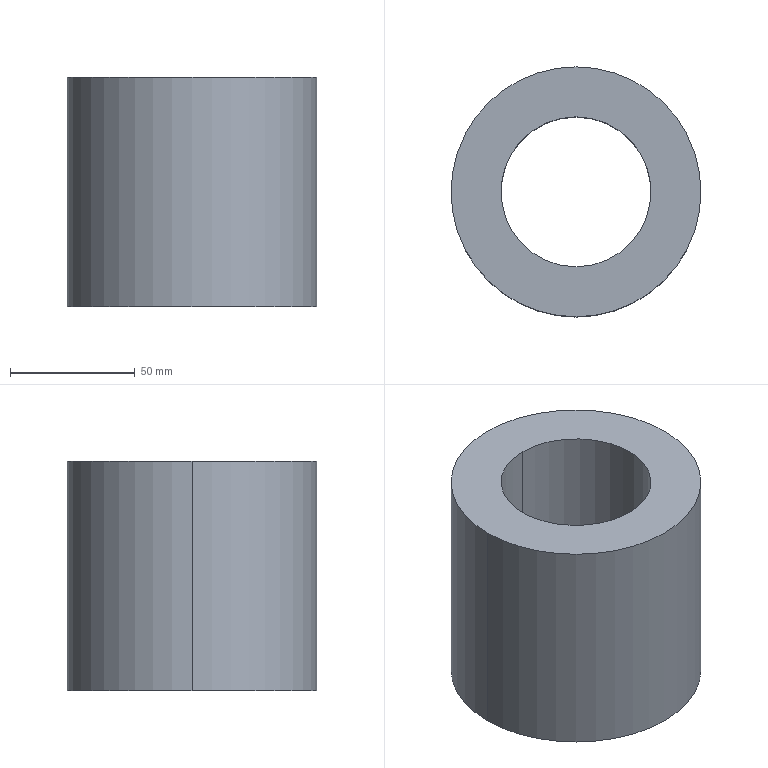Part | SolidWorks | features BaseBody 1 | 1 solid | 8 faces | box 100 x 100 x 92 mm | volume 462347 mm3 | cylinder 4 | cone 2 | plane 2 | commonest cylinder face diameters 60 x2 100 x2
STEP:
#1=CARTESIAN_POINT('',(0.,-30.,4.));
#2=VERTEX_POINT('',#1);
#3=CARTESIAN_POINT('',(0.,30.,4.));
#4=VERTEX_POINT('',#3);
#5=CARTESIAN_POINT('',(0.,0.,4.));
#6=DIRECTION('',(0.,0.,-1.));
#7=DIRECTION('',(0.,1.,0.));
#8=AXIS2_PLACEMENT_3D('',#5,#6,#7);
#9=CIRCLE('',#8,30.);
#10=EDGE_CURVE('',#2,#4,#9,.T.);
#11=ORIENTED_EDGE('',*,*,#10,.F.);
#12=CARTESIAN_POINT('',(0.,-31.,3.));
#13=VERTEX_POINT('',#12);
#14=CARTESIAN_POINT('',(0.,-30.,4.));
#15=DIRECTION('',(0.,-0.7071,-0.7071));
#16=VECTOR('',#15,1000.);
#17=LINE('',#14,#16);
#18=EDGE_CURVE('',#2,#13,#17,.T.);
#19=ORIENTED_EDGE('',*,*,#18,.T.);
#20=CARTESIAN_POINT('',(0.,31.,3.));
#21=VERTEX_POINT('',#20);
#22=CARTESIAN_POINT('',(0.,0.,3.));
#23=DIRECTION('',(0.,0.,1.));
#24=DIRECTION('',(0.,1.,0.));
#25=AXIS2_PLACEMENT_3D('',#22,#23,#24);
#26=CIRCLE('',#25,31.);
#27=EDGE_CURVE('',#21,#13,#26,.T.);
#28=ORIENTED_EDGE('',*,*,#27,.F.);
#29=CARTESIAN_POINT('',(0.,30.,4.));
#30=DIRECTION('',(0.,0.7071,-0.7071));
#31=VECTOR('',#30,1000.);
#32=LINE('',#29,#31);
#33=EDGE_CURVE('',#4,#21,#32,.T.);
#34=ORIENTED_EDGE('',*,*,#33,.F.);
#35=EDGE_LOOP('',(#11,#19,#28,#34));
#36=FACE_OUTER_BOUND('',#35,.T.);
#37=CARTESIAN_POINT('',(0.,0.,4.));
#38=DIRECTION('',(0.,0.,-1.));
#39=DIRECTION('',(0.,1.,0.));
#40=AXIS2_PLACEMENT_3D('',#37,#38,#39);
#41=CONICAL_SURFACE('',#40,30.,0.7854);
#42=ADVANCED_FACE('',(#36),#41,.F.);
#43=ORIENTED_EDGE('',*,*,#10,.T.);
#44=CARTESIAN_POINT('',(0.,30.,95.));
#45=VERTEX_POINT('',#44);
#46=CARTESIAN_POINT('',(0.,30.,-80.));
#47=DIRECTION('',(0.,0.,1.));
#48=VECTOR('',#47,1000.);
#49=LINE('',#46,#48);
#50=EDGE_CURVE('',#4,#45,#49,.T.);
#51=ORIENTED_EDGE('',*,*,#50,.T.);
#52=CARTESIAN_POINT('',(0.,-30.,95.));
#53=VERTEX_POINT('',#52);
#54=CARTESIAN_POINT('',(0.,0.,95.));
#55=DIRECTION('',(0.,0.,1.));
#56=DIRECTION('',(1.,0.,0.));
#57=AXIS2_PLACEMENT_3D('',#54,#55,#56);
#58=CIRCLE('',#57,30.);
#59=EDGE_CURVE('',#45,#53,#58,.T.);
#60=ORIENTED_EDGE('',*,*,#59,.T.);
#61=CARTESIAN_POINT('',(0.,-30.,-80.));
#62=DIRECTION('',(0.,0.,1.));
#63=VECTOR('',#62,1000.);
#64=LINE('',#61,#63);
#65=EDGE_CURVE('',#2,#53,#64,.T.);
#66=ORIENTED_EDGE('',*,*,#65,.F.);
#67=EDGE_LOOP('',(#43,#51,#60,#66));
#68=FACE_OUTER_BOUND('',#67,.T.);
#69=CARTESIAN_POINT('',(0.,0.,-80.));
#70=DIRECTION('',(0.,0.,1.));
#71=DIRECTION('',(0.,-1.,0.));
#72=AXIS2_PLACEMENT_3D('',#69,#70,#71);
#73=CYLINDRICAL_SURFACE('',#72,30.);
#74=ADVANCED_FACE('',(#68),#73,.F.);
#75=CARTESIAN_POINT('',(50.,0.,95.));
#76=VERTEX_POINT('',#75);
#77=CARTESIAN_POINT('',(-50.,0.,95.));
#78=VERTEX_POINT('',#77);
#79=CARTESIAN_POINT('',(0.,0.,95.));
#80=DIRECTION('',(0.,0.,1.));
#81=DIRECTION('',(1.,0.,0.));
#82=AXIS2_PLACEMENT_3D('',#79,#80,#81);
#83=CIRCLE('',#82,50.);
#84=EDGE_CURVE('',#76,#78,#83,.T.);
#85=ORIENTED_EDGE('',*,*,#84,.F.);
#86=CARTESIAN_POINT('',(50.,0.,3.));
#87=VERTEX_POINT('',#86);
#88=CARTESIAN_POINT('',(50.,0.,95.));
#89=DIRECTION('',(0.,0.,-1.));
#90=VECTOR('',#89,1000.);
#91=LINE('',#88,#90);
#92=EDGE_CURVE('',#76,#87,#91,.T.);
#93=ORIENTED_EDGE('',*,*,#92,.T.);
#94=CARTESIAN_POINT('',(-50.,0.,3.));
#95=VERTEX_POINT('',#94);
#96=CARTESIAN_POINT('',(0.,0.,3.));
#97=DIRECTION('',(0.,0.,-1.));
#98=DIRECTION('',(0.,1.,0.));
#99=AXIS2_PLACEMENT_3D('',#96,#97,#98);
#100=CIRCLE('',#99,50.);
#101=EDGE_CURVE('',#95,#87,#100,.T.);
#102=ORIENTED_EDGE('',*,*,#101,.F.);
#103=CARTESIAN_POINT('',(-50.,0.,95.));
#104=DIRECTION('',(0.,0.,-1.));
#105=VECTOR('',#104,1000.);
#106=LINE('',#103,#105);
#107=EDGE_CURVE('',#78,#95,#106,.T.);
#108=ORIENTED_EDGE('',*,*,#107,.F.);
#109=EDGE_LOOP('',(#85,#93,#102,#108));
#110=FACE_OUTER_BOUND('',#109,.T.);
#111=CARTESIAN_POINT('',(0.,0.,95.));
#112=DIRECTION('',(0.,0.,-1.));
#113=DIRECTION('',(-1.,0.,0.));
#114=AXIS2_PLACEMENT_3D('',#111,#112,#113);
#115=CYLINDRICAL_SURFACE('',#114,50.);
#116=ADVANCED_FACE('',(#110),#115,.T.);
#117=ORIENTED_EDGE('',*,*,#92,.F.);
#118=CARTESIAN_POINT('',(0.,0.,95.));
#119=DIRECTION('',(0.,0.,1.));
#120=DIRECTION('',(1.,0.,0.));
#121=AXIS2_PLACEMENT_3D('',#118,#119,#120);
#122=CIRCLE('',#121,50.);
#123=EDGE_CURVE('',#78,#76,#122,.T.);
#124=ORIENTED_EDGE('',*,*,#123,.F.);
#125=ORIENTED_EDGE('',*,*,#107,.T.);
#126=CARTESIAN_POINT('',(0.,0.,3.));
#127=DIRECTION('',(0.,0.,-1.));
#128=DIRECTION('',(0.,1.,0.));
#129=AXIS2_PLACEMENT_3D('',#126,#127,#128);
#130=CIRCLE('',#129,50.);
#131=EDGE_CURVE('',#87,#95,#130,.T.);
#132=ORIENTED_EDGE('',*,*,#131,.F.);
#133=EDGE_LOOP('',(#117,#124,#125,#132));
#134=FACE_OUTER_BOUND('',#133,.T.);
#135=CARTESIAN_POINT('',(0.,0.,95.));
#136=DIRECTION('',(0.,0.,-1.));
#137=DIRECTION('',(-1.,0.,0.));
#138=AXIS2_PLACEMENT_3D('',#135,#136,#137);
#139=CYLINDRICAL_SURFACE('',#138,50.);
#140=ADVANCED_FACE('',(#134),#139,.T.);
#141=CARTESIAN_POINT('',(0.,0.,95.));
#142=DIRECTION('',(0.,0.,1.));
#143=DIRECTION('',(1.,0.,0.));
#144=AXIS2_PLACEMENT_3D('',#141,#142,#143);
#145=CIRCLE('',#144,30.);
#146=EDGE_CURVE('',#53,#45,#145,.T.);
#147=ORIENTED_EDGE('',*,*,#146,.F.);
#148=ORIENTED_EDGE('',*,*,#59,.F.);
#149=EDGE_LOOP('',(#147,#148));
#150=FACE_BOUND('',#149,.T.);
#151=ORIENTED_EDGE('',*,*,#123,.T.);
#152=ORIENTED_EDGE('',*,*,#84,.T.);
#153=EDGE_LOOP('',(#151,#152));
#154=FACE_OUTER_BOUND('',#153,.T.);
#155=CARTESIAN_POINT('',(0.,0.,95.));
#156=DIRECTION('',(0.,0.,1.));
#157=DIRECTION('',(1.,0.,0.));
#158=AXIS2_PLACEMENT_3D('',#155,#156,#157);
#159=PLANE('',#158);
#160=ADVANCED_FACE('',(#150,#154),#159,.T.);
#161=ORIENTED_EDGE('',*,*,#27,.T.);
#162=CARTESIAN_POINT('',(0.,0.,3.));
#163=DIRECTION('',(0.,0.,1.));
#164=DIRECTION('',(0.,1.,0.));
#165=AXIS2_PLACEMENT_3D('',#162,#163,#164);
#166=CIRCLE('',#165,31.);
#167=EDGE_CURVE('',#13,#21,#166,.T.);
#168=ORIENTED_EDGE('',*,*,#167,.T.);
#169=EDGE_LOOP('',(#161,#168));
#170=FACE_BOUND('',#169,.T.);
#171=ORIENTED_EDGE('',*,*,#101,.T.);
#172=ORIENTED_EDGE('',*,*,#131,.T.);
#173=EDGE_LOOP('',(#171,#172));
#174=FACE_OUTER_BOUND('',#173,.T.);
#175=CARTESIAN_POINT('',(685.,0.,3.));
#176=DIRECTION('',(0.,0.,-1.));
#177=DIRECTION('',(0.,1.,0.));
#178=AXIS2_PLACEMENT_3D('',#175,#176,#177);
#179=PLANE('',#178);
#180=ADVANCED_FACE('',(#170,#174),#179,.T.);
#181=ORIENTED_EDGE('',*,*,#50,.F.);
#182=CARTESIAN_POINT('',(0.,0.,4.));
#183=DIRECTION('',(0.,0.,-1.));
#184=DIRECTION('',(0.,1.,0.));
#185=AXIS2_PLACEMENT_3D('',#182,#183,#184);
#186=CIRCLE('',#185,30.);
#187=EDGE_CURVE('',#4,#2,#186,.T.);
#188=ORIENTED_EDGE('',*,*,#187,.T.);
#189=ORIENTED_EDGE('',*,*,#65,.T.);
#190=ORIENTED_EDGE('',*,*,#146,.T.);
#191=EDGE_LOOP('',(#181,#188,#189,#190));
#192=FACE_OUTER_BOUND('',#191,.T.);
#193=CARTESIAN_POINT('',(0.,0.,-80.));
#194=DIRECTION('',(0.,0.,1.));
#195=DIRECTION('',(0.,-1.,0.));
#196=AXIS2_PLACEMENT_3D('',#193,#194,#195);
#197=CYLINDRICAL_SURFACE('',#196,30.);
#198=ADVANCED_FACE('',(#192),#197,.F.);
#199=ORIENTED_EDGE('',*,*,#18,.F.);
#200=ORIENTED_EDGE('',*,*,#187,.F.);
#201=ORIENTED_EDGE('',*,*,#33,.T.);
#202=ORIENTED_EDGE('',*,*,#167,.F.);
#203=EDGE_LOOP('',(#199,#200,#201,#202));
#204=FACE_OUTER_BOUND('',#203,.T.);
#205=CARTESIAN_POINT('',(0.,0.,4.));
#206=DIRECTION('',(0.,0.,-1.));
#207=DIRECTION('',(0.,1.,0.));
#208=AXIS2_PLACEMENT_3D('',#205,#206,#207);
#209=CONICAL_SURFACE('',#208,30.,0.7854);
#210=ADVANCED_FACE('',(#204),#209,.F.);
#211=CLOSED_SHELL('',(#42,#74,#116,#140,#160,#180,#198,#210));
#212=MANIFOLD_SOLID_BREP('',#211);
#213=CARTESIAN_POINT('',(0.,0.,0.));
#214=DIRECTION('',(0.,0.,1.));
#215=DIRECTION('',(1.,0.,0.));
#216=AXIS2_PLACEMENT_3D('',#213,#214,#215);
#217=(LENGTH_UNIT()NAMED_UNIT(*)SI_UNIT(.MILLI.,.METRE.));
#218=UNCERTAINTY_MEASURE_WITH_UNIT(LENGTH_MEASURE(0.00001),#217,'','');
#219=(NAMED_UNIT(*)PLANE_ANGLE_UNIT()SI_UNIT($,.RADIAN.));
#220=(NAMED_UNIT(*)SI_UNIT($,.STERADIAN.)SOLID_ANGLE_UNIT());
#221=(GEOMETRIC_REPRESENTATION_CONTEXT(3)GLOBAL_UNCERTAINTY_ASSIGNED_CONTEXT((#218))GLOBAL_UNIT_ASSIGNED_CONTEXT((#217,#219,#220))REPRESENTATION_CONTEXT('',''));
#222=ADVANCED_BREP_SHAPE_REPRESENTATION('',(#212,#216),#221);